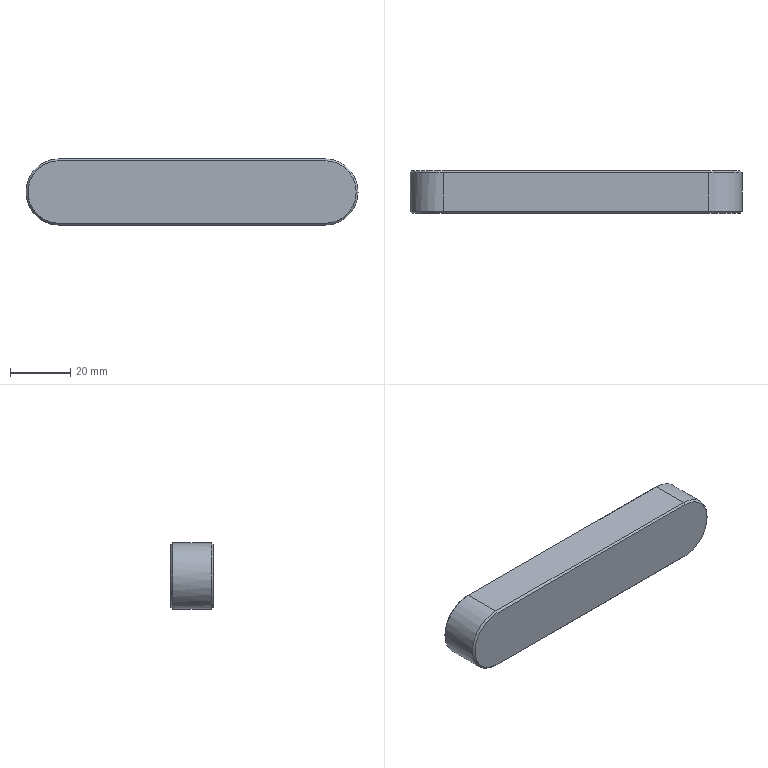Part | STEP file | Input 104 | 1 solid | 17 faces | box 110 x 14 x 22 mm | volume 32338 mm3 | plane 8 | cone 6 | cylinder 3 | commonest cylinder face diameters 22 x3
STEP:
#1=CARTESIAN_POINT('',(0.,0.,0.));
#2=DIRECTION('',(0.,0.,1.));
#3=DIRECTION('',(1.,0.,0.));
#4=AXIS2_PLACEMENT_3D('',#1,#2,#3);
#5=CARTESIAN_POINT('',(4274.4,696.,-0.4063));
#6=VERTEX_POINT('',#5);
#7=CARTESIAN_POINT('',(4264.,696.,9.994));
#8=VERTEX_POINT('',#7);
#9=CARTESIAN_POINT('',(4264.,696.,-0.4063));
#10=DIRECTION('',(0.,-1.,0.));
#11=DIRECTION('',(-1.,0.,0.));
#12=AXIS2_PLACEMENT_3D('',#9,#10,#11);
#13=CIRCLE('',#12,10.4);
#14=CARTESIAN_POINT('',(4264.,696.,-0.4063));
#15=DIRECTION('',(0.,1.,0.));
#16=DIRECTION('',(1.,0.,0.));
#17=AXIS2_PLACEMENT_3D('',#14,#15,#16);
#18=CONICAL_SURFACE('',#17,10.4,0.7854);
#19=CARTESIAN_POINT('',(9.425,0.));
#20=DIRECTION('',(-1.,0.));
#21=VECTOR('',#20,1.);
#22=LINE('',#19,#21);
#23=(GEOMETRIC_REPRESENTATION_CONTEXT(2)PARAMETRIC_REPRESENTATION_CONTEXT()REPRESENTATION_CONTEXT('',''));
#24=DEFINITIONAL_REPRESENTATION('',(#22),#23);
#25=PCURVE('',#18,#24);
#26=CARTESIAN_POINT('',(4220.,696.,-0.4063));
#27=DIRECTION('',(0.,-1.,0.));
#28=DIRECTION('',(-1.,0.,0.));
#29=AXIS2_PLACEMENT_3D('',#26,#27,#28);
#30=PLANE('',#29);
#31=CARTESIAN_POINT('',(-44.,0.));
#32=DIRECTION('',(1.,0.));
#33=AXIS2_PLACEMENT_2D('',#31,#32);
#34=CIRCLE('',#33,10.4);
#35=(GEOMETRIC_REPRESENTATION_CONTEXT(2)PARAMETRIC_REPRESENTATION_CONTEXT()REPRESENTATION_CONTEXT('',''));
#36=DEFINITIONAL_REPRESENTATION('',(#34),#35);
#37=PCURVE('',#30,#36);
#38=SURFACE_CURVE('',#13,(#25,#37),.PCURVE_S1.);
#39=EDGE_CURVE('',#6,#8,#38,.T.);
#40=ORIENTED_EDGE('',*,*,#39,.F.);
#41=CARTESIAN_POINT('',(4275.,696.6,-0.4063));
#42=VERTEX_POINT('',#41);
#43=CARTESIAN_POINT('',(4274.4,696.,-0.4063));
#44=DIRECTION('',(0.7071,0.7071,0.));
#45=VECTOR('',#44,1.);
#46=LINE('',#43,#45);
#47=CARTESIAN_POINT('',(6.283,0.));
#48=DIRECTION('',(0.,1.));
#49=VECTOR('',#48,1.);
#50=LINE('',#47,#49);
#51=(GEOMETRIC_REPRESENTATION_CONTEXT(2)PARAMETRIC_REPRESENTATION_CONTEXT()REPRESENTATION_CONTEXT('',''));
#52=DEFINITIONAL_REPRESENTATION('',(#50),#51);
#53=PCURVE('',#18,#52);
#54=CARTESIAN_POINT('',(4264.,696.,-0.4063));
#55=DIRECTION('',(0.,1.,0.));
#56=DIRECTION('',(1.,0.,0.));
#57=AXIS2_PLACEMENT_3D('',#54,#55,#56);
#58=CONICAL_SURFACE('',#57,10.4,0.7854);
#59=CARTESIAN_POINT('',(0.,0.));
#60=DIRECTION('',(0.,1.));
#61=VECTOR('',#60,1.);
#62=LINE('',#59,#61);
#63=(GEOMETRIC_REPRESENTATION_CONTEXT(2)PARAMETRIC_REPRESENTATION_CONTEXT()REPRESENTATION_CONTEXT('',''));
#64=DEFINITIONAL_REPRESENTATION('',(#62),#63);
#65=PCURVE('',#58,#64);
#66=SURFACE_CURVE('',#46,(#53,#65),.PCURVE_S1.);
#67=EDGE_CURVE('',#6,#42,#66,.T.);
#68=ORIENTED_EDGE('',*,*,#67,.T.);
#69=CARTESIAN_POINT('',(4264.,696.6,10.594));
#70=VERTEX_POINT('',#69);
#71=CARTESIAN_POINT('',(4264.,696.6,-0.4063));
#72=DIRECTION('',(0.,1.,0.));
#73=DIRECTION('',(-1.,0.,0.));
#74=AXIS2_PLACEMENT_3D('',#71,#72,#73);
#75=CIRCLE('',#74,11.);
#76=CARTESIAN_POINT('',(3.142,0.6));
#77=DIRECTION('',(1.,0.));
#78=VECTOR('',#77,1.);
#79=LINE('',#76,#78);
#80=(GEOMETRIC_REPRESENTATION_CONTEXT(2)PARAMETRIC_REPRESENTATION_CONTEXT()REPRESENTATION_CONTEXT('',''));
#81=DEFINITIONAL_REPRESENTATION('',(#79),#80);
#82=PCURVE('',#18,#81);
#83=CARTESIAN_POINT('',(4264.,696.,-0.4063));
#84=DIRECTION('',(0.,1.,0.));
#85=DIRECTION('',(1.,0.,0.));
#86=AXIS2_PLACEMENT_3D('',#83,#84,#85);
#87=CYLINDRICAL_SURFACE('',#86,11.);
#88=CARTESIAN_POINT('',(3.142,0.6));
#89=DIRECTION('',(1.,0.));
#90=VECTOR('',#89,1.);
#91=LINE('',#88,#90);
#92=(GEOMETRIC_REPRESENTATION_CONTEXT(2)PARAMETRIC_REPRESENTATION_CONTEXT()REPRESENTATION_CONTEXT('',''));
#93=DEFINITIONAL_REPRESENTATION('',(#91),#92);
#94=PCURVE('',#87,#93);
#95=SURFACE_CURVE('',#75,(#82,#94),.PCURVE_S1.);
#96=EDGE_CURVE('',#70,#42,#95,.T.);
#97=ORIENTED_EDGE('',*,*,#96,.F.);
#98=CARTESIAN_POINT('',(4264.,696.,9.994));
#99=DIRECTION('',(0.,0.7071,0.7071));
#100=VECTOR('',#99,1.);
#101=LINE('',#98,#100);
#102=CARTESIAN_POINT('',(4.712,0.));
#103=DIRECTION('',(0.,1.));
#104=VECTOR('',#103,1.);
#105=LINE('',#102,#104);
#106=(GEOMETRIC_REPRESENTATION_CONTEXT(2)PARAMETRIC_REPRESENTATION_CONTEXT()REPRESENTATION_CONTEXT('',''));
#107=DEFINITIONAL_REPRESENTATION('',(#105),#106);
#108=PCURVE('',#18,#107);
#109=CARTESIAN_POINT('',(4220.,696.6,10.594));
#110=DIRECTION('',(0.,0.7071,-0.7071));
#111=DIRECTION('',(0.,0.7071,0.7071));
#112=AXIS2_PLACEMENT_3D('',#109,#110,#111);
#113=PLANE('',#112);
#114=CARTESIAN_POINT('',(-0.8485,44.));
#115=DIRECTION('',(1.,0.));
#116=VECTOR('',#115,1.);
#117=LINE('',#114,#116);
#118=(GEOMETRIC_REPRESENTATION_CONTEXT(2)PARAMETRIC_REPRESENTATION_CONTEXT()REPRESENTATION_CONTEXT('',''));
#119=DEFINITIONAL_REPRESENTATION('',(#117),#118);
#120=PCURVE('',#113,#119);
#121=SURFACE_CURVE('',#101,(#108,#120),.PCURVE_S1.);
#122=EDGE_CURVE('',#8,#70,#121,.T.);
#123=ORIENTED_EDGE('',*,*,#122,.F.);
#124=EDGE_LOOP('',(#40,#68,#97,#123));
#125=FACE_BOUND('',#124,.T.);
#126=ADVANCED_FACE('',(#125),#18,.T.);
#127=CARTESIAN_POINT('',(4165.6,710.,-0.4063));
#128=VERTEX_POINT('',#127);
#129=CARTESIAN_POINT('',(4176.,710.,9.994));
#130=VERTEX_POINT('',#129);
#131=CARTESIAN_POINT('',(4176.,710.,-0.4063));
#132=DIRECTION('',(0.,1.,0.));
#133=DIRECTION('',(1.,0.,0.));
#134=AXIS2_PLACEMENT_3D('',#131,#132,#133);
#135=CIRCLE('',#134,10.4);
#136=CARTESIAN_POINT('',(4176.,710.,-0.4063));
#137=DIRECTION('',(0.,-1.,0.));
#138=DIRECTION('',(-1.,0.,0.));
#139=AXIS2_PLACEMENT_3D('',#136,#137,#138);
#140=CONICAL_SURFACE('',#139,10.4,0.7854);
#141=CARTESIAN_POINT('',(9.425,0.));
#142=DIRECTION('',(-1.,0.));
#143=VECTOR('',#142,1.);
#144=LINE('',#141,#143);
#145=(GEOMETRIC_REPRESENTATION_CONTEXT(2)PARAMETRIC_REPRESENTATION_CONTEXT()REPRESENTATION_CONTEXT('',''));
#146=DEFINITIONAL_REPRESENTATION('',(#144),#145);
#147=PCURVE('',#140,#146);
#148=CARTESIAN_POINT('',(4220.,710.,-0.4063));
#149=DIRECTION('',(0.,1.,0.));
#150=DIRECTION('',(1.,0.,0.));
#151=AXIS2_PLACEMENT_3D('',#148,#149,#150);
#152=PLANE('',#151);
#153=CARTESIAN_POINT('',(-44.,0.));
#154=DIRECTION('',(1.,0.));
#155=AXIS2_PLACEMENT_2D('',#153,#154);
#156=CIRCLE('',#155,10.4);
#157=(GEOMETRIC_REPRESENTATION_CONTEXT(2)PARAMETRIC_REPRESENTATION_CONTEXT()REPRESENTATION_CONTEXT('',''));
#158=DEFINITIONAL_REPRESENTATION('',(#156),#157);
#159=PCURVE('',#152,#158);
#160=SURFACE_CURVE('',#135,(#147,#159),.PCURVE_S1.);
#161=EDGE_CURVE('',#128,#130,#160,.T.);
#162=ORIENTED_EDGE('',*,*,#161,.F.);
#163=CARTESIAN_POINT('',(4165.,709.4,-0.4063));
#164=VERTEX_POINT('',#163);
#165=CARTESIAN_POINT('',(4165.6,710.,-0.4063));
#166=DIRECTION('',(-0.7071,-0.7071,0.));
#167=VECTOR('',#166,1.);
#168=LINE('',#165,#167);
#169=CARTESIAN_POINT('',(6.283,0.));
#170=DIRECTION('',(0.,1.));
#171=VECTOR('',#170,1.);
#172=LINE('',#169,#171);
#173=(GEOMETRIC_REPRESENTATION_CONTEXT(2)PARAMETRIC_REPRESENTATION_CONTEXT()REPRESENTATION_CONTEXT('',''));
#174=DEFINITIONAL_REPRESENTATION('',(#172),#173);
#175=PCURVE('',#140,#174);
#176=CARTESIAN_POINT('',(4176.,710.,-0.4063));
#177=DIRECTION('',(0.,-1.,0.));
#178=DIRECTION('',(-1.,0.,0.));
#179=AXIS2_PLACEMENT_3D('',#176,#177,#178);
#180=CONICAL_SURFACE('',#179,10.4,0.7854);
#181=CARTESIAN_POINT('',(0.,0.));
#182=DIRECTION('',(0.,1.));
#183=VECTOR('',#182,1.);
#184=LINE('',#181,#183);
#185=(GEOMETRIC_REPRESENTATION_CONTEXT(2)PARAMETRIC_REPRESENTATION_CONTEXT()REPRESENTATION_CONTEXT('',''));
#186=DEFINITIONAL_REPRESENTATION('',(#184),#185);
#187=PCURVE('',#180,#186);
#188=SURFACE_CURVE('',#168,(#175,#187),.PCURVE_S1.);
#189=EDGE_CURVE('',#128,#164,#188,.T.);
#190=ORIENTED_EDGE('',*,*,#189,.T.);
#191=CARTESIAN_POINT('',(4176.,709.4,10.594));
#192=VERTEX_POINT('',#191);
#193=CARTESIAN_POINT('',(4176.,709.4,-0.4063));
#194=DIRECTION('',(0.,-1.,0.));
#195=DIRECTION('',(1.,0.,0.));
#196=AXIS2_PLACEMENT_3D('',#193,#194,#195);
#197=CIRCLE('',#196,11.);
#198=CARTESIAN_POINT('',(3.142,0.6));
#199=DIRECTION('',(1.,0.));
#200=VECTOR('',#199,1.);
#201=LINE('',#198,#200);
#202=(GEOMETRIC_REPRESENTATION_CONTEXT(2)PARAMETRIC_REPRESENTATION_CONTEXT()REPRESENTATION_CONTEXT('',''));
#203=DEFINITIONAL_REPRESENTATION('',(#201),#202);
#204=PCURVE('',#140,#203);
#205=CARTESIAN_POINT('',(4176.,696.,-0.4063));
#206=DIRECTION('',(0.,1.,0.));
#207=DIRECTION('',(1.,0.,0.));
#208=AXIS2_PLACEMENT_3D('',#205,#206,#207);
#209=CYLINDRICAL_SURFACE('',#208,11.);
#210=CARTESIAN_POINT('',(6.283,13.4));
#211=DIRECTION('',(-1.,0.));
#212=VECTOR('',#211,1.);
#213=LINE('',#210,#212);
#214=(GEOMETRIC_REPRESENTATION_CONTEXT(2)PARAMETRIC_REPRESENTATION_CONTEXT()REPRESENTATION_CONTEXT('',''));
#215=DEFINITIONAL_REPRESENTATION('',(#213),#214);
#216=PCURVE('',#209,#215);
#217=SURFACE_CURVE('',#197,(#204,#216),.PCURVE_S1.);
#218=EDGE_CURVE('',#192,#164,#217,.T.);
#219=ORIENTED_EDGE('',*,*,#218,.F.);
#220=CARTESIAN_POINT('',(4176.,709.4,10.594));
#221=DIRECTION('',(0.,0.7071,-0.7071));
#222=VECTOR('',#221,1.);
#223=LINE('',#220,#222);
#224=CARTESIAN_POINT('',(4.712,0.6));
#225=DIRECTION('',(0.,-1.));
#226=VECTOR('',#225,1.);
#227=LINE('',#224,#226);
#228=(GEOMETRIC_REPRESENTATION_CONTEXT(2)PARAMETRIC_REPRESENTATION_CONTEXT()REPRESENTATION_CONTEXT('',''));
#229=DEFINITIONAL_REPRESENTATION('',(#227),#228);
#230=PCURVE('',#140,#229);
#231=CARTESIAN_POINT('',(4220.,709.4,10.594));
#232=DIRECTION('',(0.,-0.7071,-0.7071));
#233=DIRECTION('',(0.,0.7071,-0.7071));
#234=AXIS2_PLACEMENT_3D('',#231,#232,#233);
#235=PLANE('',#234);
#236=CARTESIAN_POINT('',(0.,-44.));
#237=DIRECTION('',(1.,0.));
#238=VECTOR('',#237,1.);
#239=LINE('',#236,#238);
#240=(GEOMETRIC_REPRESENTATION_CONTEXT(2)PARAMETRIC_REPRESENTATION_CONTEXT()REPRESENTATION_CONTEXT('',''));
#241=DEFINITIONAL_REPRESENTATION('',(#239),#240);
#242=PCURVE('',#235,#241);
#243=SURFACE_CURVE('',#223,(#230,#242),.PCURVE_S1.);
#244=EDGE_CURVE('',#192,#130,#243,.T.);
#245=ORIENTED_EDGE('',*,*,#244,.T.);
#246=EDGE_LOOP('',(#162,#190,#219,#245));
#247=FACE_BOUND('',#246,.T.);
#248=ADVANCED_FACE('',(#247),#140,.T.);
#249=ORIENTED_EDGE('',*,*,#96,.T.);
#250=CARTESIAN_POINT('',(4275.,709.4,-0.4063));
#251=VERTEX_POINT('',#250);
#252=CARTESIAN_POINT('',(4275.,696.,-0.4063));
#253=DIRECTION('',(0.,1.,0.));
#254=VECTOR('',#253,1.);
#255=LINE('',#252,#254);
#256=CARTESIAN_POINT('',(6.283,0.));
#257=DIRECTION('',(0.,1.));
#258=VECTOR('',#257,1.);
#259=LINE('',#256,#258);
#260=(GEOMETRIC_REPRESENTATION_CONTEXT(2)PARAMETRIC_REPRESENTATION_CONTEXT()REPRESENTATION_CONTEXT('',''));
#261=DEFINITIONAL_REPRESENTATION('',(#259),#260);
#262=PCURVE('',#87,#261);
#263=CARTESIAN_POINT('',(4264.,696.,-0.4063));
#264=DIRECTION('',(0.,1.,0.));
#265=DIRECTION('',(1.,0.,0.));
#266=AXIS2_PLACEMENT_3D('',#263,#264,#265);
#267=CYLINDRICAL_SURFACE('',#266,11.);
#268=CARTESIAN_POINT('',(0.,0.));
#269=DIRECTION('',(0.,1.));
#270=VECTOR('',#269,1.);
#271=LINE('',#268,#270);
#272=(GEOMETRIC_REPRESENTATION_CONTEXT(2)PARAMETRIC_REPRESENTATION_CONTEXT()REPRESENTATION_CONTEXT('',''));
#273=DEFINITIONAL_REPRESENTATION('',(#271),#272);
#274=PCURVE('',#267,#273);
#275=SURFACE_CURVE('',#255,(#262,#274),.PCURVE_S1.);
#276=EDGE_CURVE('',#42,#251,#275,.T.);
#277=ORIENTED_EDGE('',*,*,#276,.T.);
#278=CARTESIAN_POINT('',(4264.,709.4,10.594));
#279=VERTEX_POINT('',#278);
#280=CARTESIAN_POINT('',(4264.,709.4,-0.4063));
#281=DIRECTION('',(0.,-1.,0.));
#282=DIRECTION('',(1.,0.,0.));
#283=AXIS2_PLACEMENT_3D('',#280,#281,#282);
#284=CIRCLE('',#283,11.);
#285=CARTESIAN_POINT('',(6.283,13.4));
#286=DIRECTION('',(-1.,0.));
#287=VECTOR('',#286,1.);
#288=LINE('',#285,#287);
#289=(GEOMETRIC_REPRESENTATION_CONTEXT(2)PARAMETRIC_REPRESENTATION_CONTEXT()REPRESENTATION_CONTEXT('',''));
#290=DEFINITIONAL_REPRESENTATION('',(#288),#289);
#291=PCURVE('',#87,#290);
#292=CARTESIAN_POINT('',(4264.,710.,-0.4063));
#293=DIRECTION('',(0.,-1.,0.));
#294=DIRECTION('',(-1.,0.,0.));
#295=AXIS2_PLACEMENT_3D('',#292,#293,#294);
#296=CONICAL_SURFACE('',#295,10.4,0.7854);
#297=CARTESIAN_POINT('',(3.142,0.6));
#298=DIRECTION('',(1.,0.));
#299=VECTOR('',#298,1.);
#300=LINE('',#297,#299);
#301=(GEOMETRIC_REPRESENTATION_CONTEXT(2)PARAMETRIC_REPRESENTATION_CONTEXT()REPRESENTATION_CONTEXT('',''));
#302=DEFINITIONAL_REPRESENTATION('',(#300),#301);
#303=PCURVE('',#296,#302);
#304=SURFACE_CURVE('',#284,(#291,#303),.PCURVE_S1.);
#305=EDGE_CURVE('',#251,#279,#304,.T.);
#306=ORIENTED_EDGE('',*,*,#305,.T.);
#307=CARTESIAN_POINT('',(4264.,696.,10.594));
#308=DIRECTION('',(0.,1.,0.));
#309=VECTOR('',#308,1.);
#310=LINE('',#307,#309);
#311=CARTESIAN_POINT('',(4.712,0.));
#312=DIRECTION('',(0.,1.));
#313=VECTOR('',#312,1.);
#314=LINE('',#311,#313);
#315=(GEOMETRIC_REPRESENTATION_CONTEXT(2)PARAMETRIC_REPRESENTATION_CONTEXT()REPRESENTATION_CONTEXT('',''));
#316=DEFINITIONAL_REPRESENTATION('',(#314),#315);
#317=PCURVE('',#87,#316);
#318=CARTESIAN_POINT('',(4220.,696.,10.594));
#319=DIRECTION('',(0.,0.,1.));
#320=DIRECTION('',(0.,-1.,0.));
#321=AXIS2_PLACEMENT_3D('',#318,#319,#320);
#322=PLANE('',#321);
#323=CARTESIAN_POINT('',(0.,44.));
#324=DIRECTION('',(-1.,0.));
#325=VECTOR('',#324,1.);
#326=LINE('',#323,#325);
#327=(GEOMETRIC_REPRESENTATION_CONTEXT(2)PARAMETRIC_REPRESENTATION_CONTEXT()REPRESENTATION_CONTEXT('',''));
#328=DEFINITIONAL_REPRESENTATION('',(#326),#327);
#329=PCURVE('',#322,#328);
#330=SURFACE_CURVE('',#310,(#317,#329),.PCURVE_S1.);
#331=EDGE_CURVE('',#70,#279,#330,.T.);
#332=ORIENTED_EDGE('',*,*,#331,.F.);
#333=EDGE_LOOP('',(#249,#277,#306,#332));
#334=FACE_BOUND('',#333,.T.);
#335=ADVANCED_FACE('',(#334),#87,.T.);
#336=CARTESIAN_POINT('',(4264.,710.,-10.806));
#337=VERTEX_POINT('',#336);
#338=CARTESIAN_POINT('',(4176.,710.,-10.806));
#339=VERTEX_POINT('',#338);
#340=CARTESIAN_POINT('',(4220.,710.,-10.806));
#341=DIRECTION('',(-1.,0.,0.));
#342=VECTOR('',#341,1.);
#343=LINE('',#340,#342);
#344=CARTESIAN_POINT('',(0.,10.4));
#345=DIRECTION('',(-1.,0.));
#346=VECTOR('',#345,1.);
#347=LINE('',#344,#346);
#348=(GEOMETRIC_REPRESENTATION_CONTEXT(2)PARAMETRIC_REPRESENTATION_CONTEXT()REPRESENTATION_CONTEXT('',''));
#349=DEFINITIONAL_REPRESENTATION('',(#347),#348);
#350=PCURVE('',#152,#349);
#351=CARTESIAN_POINT('',(4220.,709.4,-11.406));
#352=DIRECTION('',(0.,-0.7071,0.7071));
#353=DIRECTION('',(0.,-0.7071,-0.7071));
#354=AXIS2_PLACEMENT_3D('',#351,#352,#353);
#355=PLANE('',#354);
#356=CARTESIAN_POINT('',(-0.8485,0.));
#357=DIRECTION('',(0.,-1.));
#358=VECTOR('',#357,1.);
#359=LINE('',#356,#358);
#360=(GEOMETRIC_REPRESENTATION_CONTEXT(2)PARAMETRIC_REPRESENTATION_CONTEXT()REPRESENTATION_CONTEXT('',''));
#361=DEFINITIONAL_REPRESENTATION('',(#359),#360);
#362=PCURVE('',#355,#361);
#363=SURFACE_CURVE('',#343,(#350,#362),.PCURVE_S1.);
#364=EDGE_CURVE('',#337,#339,#363,.T.);
#365=ORIENTED_EDGE('',*,*,#364,.T.);
#366=CARTESIAN_POINT('',(4176.,710.,-0.4063));
#367=DIRECTION('',(0.,1.,0.));
#368=DIRECTION('',(1.,0.,0.));
#369=AXIS2_PLACEMENT_3D('',#366,#367,#368);
#370=CIRCLE('',#369,10.4);
#371=CARTESIAN_POINT('',(-44.,0.));
#372=DIRECTION('',(1.,0.));
#373=AXIS2_PLACEMENT_2D('',#371,#372);
#374=CIRCLE('',#373,10.4);
#375=(GEOMETRIC_REPRESENTATION_CONTEXT(2)PARAMETRIC_REPRESENTATION_CONTEXT()REPRESENTATION_CONTEXT('',''));
#376=DEFINITIONAL_REPRESENTATION('',(#374),#375);
#377=PCURVE('',#152,#376);
#378=CARTESIAN_POINT('',(3.142,0.));
#379=DIRECTION('',(-1.,0.));
#380=VECTOR('',#379,1.);
#381=LINE('',#378,#380);
#382=(GEOMETRIC_REPRESENTATION_CONTEXT(2)PARAMETRIC_REPRESENTATION_CONTEXT()REPRESENTATION_CONTEXT('',''));
#383=DEFINITIONAL_REPRESENTATION('',(#381),#382);
#384=PCURVE('',#180,#383);
#385=SURFACE_CURVE('',#370,(#377,#384),.PCURVE_S1.);
#386=EDGE_CURVE('',#339,#128,#385,.T.);
#387=ORIENTED_EDGE('',*,*,#386,.T.);
#388=ORIENTED_EDGE('',*,*,#161,.T.);
#389=CARTESIAN_POINT('',(4264.,710.,9.994));
#390=VERTEX_POINT('',#389);
#391=CARTESIAN_POINT('',(4220.,710.,9.994));
#392=DIRECTION('',(1.,0.,0.));
#393=VECTOR('',#392,1.);
#394=LINE('',#391,#393);
#395=CARTESIAN_POINT('',(0.,-10.4));
#396=DIRECTION('',(1.,0.));
#397=VECTOR('',#396,1.);
#398=LINE('',#395,#397);
#399=(GEOMETRIC_REPRESENTATION_CONTEXT(2)PARAMETRIC_REPRESENTATION_CONTEXT()REPRESENTATION_CONTEXT('',''));
#400=DEFINITIONAL_REPRESENTATION('',(#398),#399);
#401=PCURVE('',#152,#400);
#402=CARTESIAN_POINT('',(0.8485,0.));
#403=DIRECTION('',(0.,1.));
#404=VECTOR('',#403,1.);
#405=LINE('',#402,#404);
#406=(GEOMETRIC_REPRESENTATION_CONTEXT(2)PARAMETRIC_REPRESENTATION_CONTEXT()REPRESENTATION_CONTEXT('',''));
#407=DEFINITIONAL_REPRESENTATION('',(#405),#406);
#408=PCURVE('',#235,#407);
#409=SURFACE_CURVE('',#394,(#401,#408),.PCURVE_S1.);
#410=EDGE_CURVE('',#130,#390,#409,.T.);
#411=ORIENTED_EDGE('',*,*,#410,.T.);
#412=CARTESIAN_POINT('',(4264.,710.,-0.4063));
#413=DIRECTION('',(0.,1.,0.));
#414=DIRECTION('',(1.,0.,0.));
#415=AXIS2_PLACEMENT_3D('',#412,#413,#414);
#416=CIRCLE('',#415,10.4);
#417=CARTESIAN_POINT('',(44.,0.));
#418=DIRECTION('',(1.,0.));
#419=AXIS2_PLACEMENT_2D('',#417,#418);
#420=CIRCLE('',#419,10.4);
#421=(GEOMETRIC_REPRESENTATION_CONTEXT(2)PARAMETRIC_REPRESENTATION_CONTEXT()REPRESENTATION_CONTEXT('',''));
#422=DEFINITIONAL_REPRESENTATION('',(#420),#421);
#423=PCURVE('',#152,#422);
#424=CARTESIAN_POINT('',(9.425,0.));
#425=DIRECTION('',(-1.,0.));
#426=VECTOR('',#425,1.);
#427=LINE('',#424,#426);
#428=(GEOMETRIC_REPRESENTATION_CONTEXT(2)PARAMETRIC_REPRESENTATION_CONTEXT()REPRESENTATION_CONTEXT('',''));
#429=DEFINITIONAL_REPRESENTATION('',(#427),#428);
#430=PCURVE('',#296,#429);
#431=SURFACE_CURVE('',#416,(#423,#430),.PCURVE_S1.);
#432=EDGE_CURVE('',#390,#337,#431,.T.);
#433=ORIENTED_EDGE('',*,*,#432,.T.);
#434=EDGE_LOOP('',(#365,#387,#388,#411,#433));
#435=FACE_BOUND('',#434,.T.);
#436=ADVANCED_FACE('',(#435),#152,.T.);
#437=CARTESIAN_POINT('',(4176.,696.6,10.594));
#438=VERTEX_POINT('',#437);
#439=CARTESIAN_POINT('',(4176.,696.,10.594));
#440=DIRECTION('',(0.,-1.,0.));
#441=VECTOR('',#440,1.);
#442=LINE('',#439,#441);
#443=CARTESIAN_POINT('',(0.,-44.));
#444=DIRECTION('',(1.,0.));
#445=VECTOR('',#444,1.);
#446=LINE('',#443,#445);
#447=(GEOMETRIC_REPRESENTATION_CONTEXT(2)PARAMETRIC_REPRESENTATION_CONTEXT()REPRESENTATION_CONTEXT('',''));
#448=DEFINITIONAL_REPRESENTATION('',(#446),#447);
#449=PCURVE('',#322,#448);
#450=CARTESIAN_POINT('',(4.712,0.));
#451=DIRECTION('',(0.,-1.));
#452=VECTOR('',#451,1.);
#453=LINE('',#450,#452);
#454=(GEOMETRIC_REPRESENTATION_CONTEXT(2)PARAMETRIC_REPRESENTATION_CONTEXT()REPRESENTATION_CONTEXT('',''));
#455=DEFINITIONAL_REPRESENTATION('',(#453),#454);
#456=PCURVE('',#209,#455);
#457=SURFACE_CURVE('',#442,(#449,#456),.PCURVE_S1.);
#458=EDGE_CURVE('',#192,#438,#457,.T.);
#459=ORIENTED_EDGE('',*,*,#458,.T.);
#460=CARTESIAN_POINT('',(4220.,696.6,10.594));
#461=DIRECTION('',(1.,0.,0.));
#462=VECTOR('',#461,1.);
#463=LINE('',#460,#462);
#464=CARTESIAN_POINT('',(-0.6,0.));
#465=DIRECTION('',(0.,1.));
#466=VECTOR('',#465,1.);
#467=LINE('',#464,#466);
#468=(GEOMETRIC_REPRESENTATION_CONTEXT(2)PARAMETRIC_REPRESENTATION_CONTEXT()REPRESENTATION_CONTEXT('',''));
#469=DEFINITIONAL_REPRESENTATION('',(#467),#468);
#470=PCURVE('',#322,#469);
#471=CARTESIAN_POINT('',(0.,0.));
#472=DIRECTION('',(0.,1.));
#473=VECTOR('',#472,1.);
#474=LINE('',#471,#473);
#475=(GEOMETRIC_REPRESENTATION_CONTEXT(2)PARAMETRIC_REPRESENTATION_CONTEXT()REPRESENTATION_CONTEXT('',''));
#476=DEFINITIONAL_REPRESENTATION('',(#474),#475);
#477=PCURVE('',#113,#476);
#478=SURFACE_CURVE('',#463,(#470,#477),.PCURVE_S1.);
#479=EDGE_CURVE('',#438,#70,#478,.T.);
#480=ORIENTED_EDGE('',*,*,#479,.T.);
#481=ORIENTED_EDGE('',*,*,#331,.T.);
#482=CARTESIAN_POINT('',(4220.,709.4,10.594));
#483=DIRECTION('',(-1.,0.,0.));
#484=VECTOR('',#483,1.);
#485=LINE('',#482,#484);
#486=CARTESIAN_POINT('',(-13.4,0.));
#487=DIRECTION('',(0.,-1.));
#488=VECTOR('',#487,1.);
#489=LINE('',#486,#488);
#490=(GEOMETRIC_REPRESENTATION_CONTEXT(2)PARAMETRIC_REPRESENTATION_CONTEXT()REPRESENTATION_CONTEXT('',''));
#491=DEFINITIONAL_REPRESENTATION('',(#489),#490);
#492=PCURVE('',#322,#491);
#493=CARTESIAN_POINT('',(0.,0.));
#494=DIRECTION('',(0.,-1.));
#495=VECTOR('',#494,1.);
#496=LINE('',#493,#495);
#497=(GEOMETRIC_REPRESENTATION_CONTEXT(2)PARAMETRIC_REPRESENTATION_CONTEXT()REPRESENTATION_CONTEXT('',''));
#498=DEFINITIONAL_REPRESENTATION('',(#496),#497);
#499=PCURVE('',#235,#498);
#500=SURFACE_CURVE('',#485,(#492,#499),.PCURVE_S1.);
#501=EDGE_CURVE('',#279,#192,#500,.T.);
#502=ORIENTED_EDGE('',*,*,#501,.T.);
#503=EDGE_LOOP('',(#459,#480,#481,#502));
#504=FACE_BOUND('',#503,.T.);
#505=ADVANCED_FACE('',(#504),#322,.T.);
#506=CARTESIAN_POINT('',(4264.,709.4,-11.406));
#507=VERTEX_POINT('',#506);
#508=CARTESIAN_POINT('',(4264.,696.6,-11.406));
#509=VERTEX_POINT('',#508);
#510=CARTESIAN_POINT('',(4264.,696.,-11.406));
#511=DIRECTION('',(0.,-1.,0.));
#512=VECTOR('',#511,1.);
#513=LINE('',#510,#512);
#514=CARTESIAN_POINT('',(4220.,696.,-11.406));
#515=DIRECTION('',(0.,0.,-1.));
#516=DIRECTION('',(0.,1.,0.));
#517=AXIS2_PLACEMENT_3D('',#514,#515,#516);
#518=PLANE('',#517);
#519=CARTESIAN_POINT('',(0.,44.));
#520=DIRECTION('',(-1.,0.));
#521=VECTOR('',#520,1.);
#522=LINE('',#519,#521);
#523=(GEOMETRIC_REPRESENTATION_CONTEXT(2)PARAMETRIC_REPRESENTATION_CONTEXT()REPRESENTATION_CONTEXT('',''));
#524=DEFINITIONAL_REPRESENTATION('',(#522),#523);
#525=PCURVE('',#518,#524);
#526=CARTESIAN_POINT('',(1.571,0.));
#527=DIRECTION('',(0.,-1.));
#528=VECTOR('',#527,1.);
#529=LINE('',#526,#528);
#530=(GEOMETRIC_REPRESENTATION_CONTEXT(2)PARAMETRIC_REPRESENTATION_CONTEXT()REPRESENTATION_CONTEXT('',''));
#531=DEFINITIONAL_REPRESENTATION('',(#529),#530);
#532=PCURVE('',#267,#531);
#533=SURFACE_CURVE('',#513,(#525,#532),.PCURVE_S1.);
#534=EDGE_CURVE('',#507,#509,#533,.T.);
#535=ORIENTED_EDGE('',*,*,#534,.T.);
#536=CARTESIAN_POINT('',(4176.,696.6,-11.406));
#537=VERTEX_POINT('',#536);
#538=CARTESIAN_POINT('',(4220.,696.6,-11.406));
#539=DIRECTION('',(-1.,0.,0.));
#540=VECTOR('',#539,1.);
#541=LINE('',#538,#540);
#542=CARTESIAN_POINT('',(0.6,0.));
#543=DIRECTION('',(0.,-1.));
#544=VECTOR('',#543,1.);
#545=LINE('',#542,#544);
#546=(GEOMETRIC_REPRESENTATION_CONTEXT(2)PARAMETRIC_REPRESENTATION_CONTEXT()REPRESENTATION_CONTEXT('',''));
#547=DEFINITIONAL_REPRESENTATION('',(#545),#546);
#548=PCURVE('',#518,#547);
#549=CARTESIAN_POINT('',(4220.,696.6,-11.406));
#550=DIRECTION('',(0.,0.7071,0.7071));
#551=DIRECTION('',(0.,-0.7071,0.7071));
#552=AXIS2_PLACEMENT_3D('',#549,#550,#551);
#553=PLANE('',#552);
#554=CARTESIAN_POINT('',(0.,0.));
#555=DIRECTION('',(0.,-1.));
#556=VECTOR('',#555,1.);
#557=LINE('',#554,#556);
#558=(GEOMETRIC_REPRESENTATION_CONTEXT(2)PARAMETRIC_REPRESENTATION_CONTEXT()REPRESENTATION_CONTEXT('',''));
#559=DEFINITIONAL_REPRESENTATION('',(#557),#558);
#560=PCURVE('',#553,#559);
#561=SURFACE_CURVE('',#541,(#548,#560),.PCURVE_S1.);
#562=EDGE_CURVE('',#509,#537,#561,.T.);
#563=ORIENTED_EDGE('',*,*,#562,.T.);
#564=CARTESIAN_POINT('',(4176.,709.4,-11.406));
#565=VERTEX_POINT('',#564);
#566=CARTESIAN_POINT('',(4176.,696.,-11.406));
#567=DIRECTION('',(0.,1.,0.));
#568=VECTOR('',#567,1.);
#569=LINE('',#566,#568);
#570=CARTESIAN_POINT('',(0.,-44.));
#571=DIRECTION('',(1.,0.));
#572=VECTOR('',#571,1.);
#573=LINE('',#570,#572);
#574=(GEOMETRIC_REPRESENTATION_CONTEXT(2)PARAMETRIC_REPRESENTATION_CONTEXT()REPRESENTATION_CONTEXT('',''));
#575=DEFINITIONAL_REPRESENTATION('',(#573),#574);
#576=PCURVE('',#518,#575);
#577=CARTESIAN_POINT('',(1.571,0.));
#578=DIRECTION('',(0.,1.));
#579=VECTOR('',#578,1.);
#580=LINE('',#577,#579);
#581=(GEOMETRIC_REPRESENTATION_CONTEXT(2)PARAMETRIC_REPRESENTATION_CONTEXT()REPRESENTATION_CONTEXT('',''));
#582=DEFINITIONAL_REPRESENTATION('',(#580),#581);
#583=PCURVE('',#209,#582);
#584=SURFACE_CURVE('',#569,(#576,#583),.PCURVE_S1.);
#585=EDGE_CURVE('',#537,#565,#584,.T.);
#586=ORIENTED_EDGE('',*,*,#585,.T.);
#587=CARTESIAN_POINT('',(4220.,709.4,-11.406));
#588=DIRECTION('',(1.,0.,0.));
#589=VECTOR('',#588,1.);
#590=LINE('',#587,#589);
#591=CARTESIAN_POINT('',(13.4,0.));
#592=DIRECTION('',(0.,1.));
#593=VECTOR('',#592,1.);
#594=LINE('',#591,#593);
#595=(GEOMETRIC_REPRESENTATION_CONTEXT(2)PARAMETRIC_REPRESENTATION_CONTEXT()REPRESENTATION_CONTEXT('',''));
#596=DEFINITIONAL_REPRESENTATION('',(#594),#595);
#597=PCURVE('',#518,#596);
#598=CARTESIAN_POINT('',(0.,0.));
#599=DIRECTION('',(0.,1.));
#600=VECTOR('',#599,1.);
#601=LINE('',#598,#600);
#602=(GEOMETRIC_REPRESENTATION_CONTEXT(2)PARAMETRIC_REPRESENTATION_CONTEXT()REPRESENTATION_CONTEXT('',''));
#603=DEFINITIONAL_REPRESENTATION('',(#601),#602);
#604=PCURVE('',#355,#603);
#605=SURFACE_CURVE('',#590,(#597,#604),.PCURVE_S1.);
#606=EDGE_CURVE('',#565,#507,#605,.T.);
#607=ORIENTED_EDGE('',*,*,#606,.T.);
#608=EDGE_LOOP('',(#535,#563,#586,#607));
#609=FACE_BOUND('',#608,.T.);
#610=ADVANCED_FACE('',(#609),#518,.T.);
#611=CARTESIAN_POINT('',(4176.,696.,9.994));
#612=VERTEX_POINT('',#611);
#613=CARTESIAN_POINT('',(4220.,696.,9.994));
#614=DIRECTION('',(-1.,0.,0.));
#615=VECTOR('',#614,1.);
#616=LINE('',#613,#615);
#617=CARTESIAN_POINT('',(0.,-10.4));
#618=DIRECTION('',(1.,0.));
#619=VECTOR('',#618,1.);
#620=LINE('',#617,#619);
#621=(GEOMETRIC_REPRESENTATION_CONTEXT(2)PARAMETRIC_REPRESENTATION_CONTEXT()REPRESENTATION_CONTEXT('',''));
#622=DEFINITIONAL_REPRESENTATION('',(#620),#621);
#623=PCURVE('',#30,#622);
#624=CARTESIAN_POINT('',(-0.8485,0.));
#625=DIRECTION('',(0.,-1.));
#626=VECTOR('',#625,1.);
#627=LINE('',#624,#626);
#628=(GEOMETRIC_REPRESENTATION_CONTEXT(2)PARAMETRIC_REPRESENTATION_CONTEXT()REPRESENTATION_CONTEXT('',''));
#629=DEFINITIONAL_REPRESENTATION('',(#627),#628);
#630=PCURVE('',#113,#629);
#631=SURFACE_CURVE('',#616,(#623,#630),.PCURVE_S1.);
#632=EDGE_CURVE('',#8,#612,#631,.T.);
#633=ORIENTED_EDGE('',*,*,#632,.T.);
#634=CARTESIAN_POINT('',(4176.,696.,-10.806));
#635=VERTEX_POINT('',#634);
#636=CARTESIAN_POINT('',(4176.,696.,-0.4063));
#637=DIRECTION('',(0.,-1.,0.));
#638=DIRECTION('',(-1.,0.,0.));
#639=AXIS2_PLACEMENT_3D('',#636,#637,#638);
#640=CIRCLE('',#639,10.4);
#641=CARTESIAN_POINT('',(44.,0.));
#642=DIRECTION('',(1.,0.));
#643=AXIS2_PLACEMENT_2D('',#641,#642);
#644=CIRCLE('',#643,10.4);
#645=(GEOMETRIC_REPRESENTATION_CONTEXT(2)PARAMETRIC_REPRESENTATION_CONTEXT()REPRESENTATION_CONTEXT('',''));
#646=DEFINITIONAL_REPRESENTATION('',(#644),#645);
#647=PCURVE('',#30,#646);
#648=CARTESIAN_POINT('',(4176.,696.,-0.4063));
#649=DIRECTION('',(0.,1.,0.));
#650=DIRECTION('',(1.,0.,0.));
#651=AXIS2_PLACEMENT_3D('',#648,#649,#650);
#652=CONICAL_SURFACE('',#651,10.4,0.7854);
#653=CARTESIAN_POINT('',(9.425,0.));
#654=DIRECTION('',(-1.,0.));
#655=VECTOR('',#654,1.);
#656=LINE('',#653,#655);
#657=(GEOMETRIC_REPRESENTATION_CONTEXT(2)PARAMETRIC_REPRESENTATION_CONTEXT()REPRESENTATION_CONTEXT('',''));
#658=DEFINITIONAL_REPRESENTATION('',(#656),#657);
#659=PCURVE('',#652,#658);
#660=SURFACE_CURVE('',#640,(#647,#659),.PCURVE_S1.);
#661=EDGE_CURVE('',#612,#635,#660,.T.);
#662=ORIENTED_EDGE('',*,*,#661,.T.);
#663=CARTESIAN_POINT('',(4264.,696.,-10.806));
#664=VERTEX_POINT('',#663);
#665=CARTESIAN_POINT('',(4220.,696.,-10.806));
#666=DIRECTION('',(1.,0.,0.));
#667=VECTOR('',#666,1.);
#668=LINE('',#665,#667);
#669=CARTESIAN_POINT('',(0.,10.4));
#670=DIRECTION('',(-1.,0.));
#671=VECTOR('',#670,1.);
#672=LINE('',#669,#671);
#673=(GEOMETRIC_REPRESENTATION_CONTEXT(2)PARAMETRIC_REPRESENTATION_CONTEXT()REPRESENTATION_CONTEXT('',''));
#674=DEFINITIONAL_REPRESENTATION('',(#672),#673);
#675=PCURVE('',#30,#674);
#676=CARTESIAN_POINT('',(0.8485,0.));
#677=DIRECTION('',(0.,1.));
#678=VECTOR('',#677,1.);
#679=LINE('',#676,#678);
#680=(GEOMETRIC_REPRESENTATION_CONTEXT(2)PARAMETRIC_REPRESENTATION_CONTEXT()REPRESENTATION_CONTEXT('',''));
#681=DEFINITIONAL_REPRESENTATION('',(#679),#680);
#682=PCURVE('',#553,#681);
#683=SURFACE_CURVE('',#668,(#675,#682),.PCURVE_S1.);
#684=EDGE_CURVE('',#635,#664,#683,.T.);
#685=ORIENTED_EDGE('',*,*,#684,.T.);
#686=CARTESIAN_POINT('',(4264.,696.,-0.4063));
#687=DIRECTION('',(0.,-1.,0.));
#688=DIRECTION('',(-1.,0.,0.));
#689=AXIS2_PLACEMENT_3D('',#686,#687,#688);
#690=CIRCLE('',#689,10.4);
#691=CARTESIAN_POINT('',(-44.,0.));
#692=DIRECTION('',(1.,0.));
#693=AXIS2_PLACEMENT_2D('',#691,#692);
#694=CIRCLE('',#693,10.4);
#695=(GEOMETRIC_REPRESENTATION_CONTEXT(2)PARAMETRIC_REPRESENTATION_CONTEXT()REPRESENTATION_CONTEXT('',''));
#696=DEFINITIONAL_REPRESENTATION('',(#694),#695);
#697=PCURVE('',#30,#696);
#698=CARTESIAN_POINT('',(3.142,0.));
#699=DIRECTION('',(-1.,0.));
#700=VECTOR('',#699,1.);
#701=LINE('',#698,#700);
#702=(GEOMETRIC_REPRESENTATION_CONTEXT(2)PARAMETRIC_REPRESENTATION_CONTEXT()REPRESENTATION_CONTEXT('',''));
#703=DEFINITIONAL_REPRESENTATION('',(#701),#702);
#704=PCURVE('',#58,#703);
#705=SURFACE_CURVE('',#690,(#697,#704),.PCURVE_S1.);
#706=EDGE_CURVE('',#664,#6,#705,.T.);
#707=ORIENTED_EDGE('',*,*,#706,.T.);
#708=ORIENTED_EDGE('',*,*,#39,.T.);
#709=EDGE_LOOP('',(#633,#662,#685,#707,#708));
#710=FACE_BOUND('',#709,.T.);
#711=ADVANCED_FACE('',(#710),#30,.T.);
#712=ORIENTED_EDGE('',*,*,#276,.F.);
#713=CARTESIAN_POINT('',(4264.,696.6,-0.4063));
#714=DIRECTION('',(0.,1.,0.));
#715=DIRECTION('',(-1.,0.,0.));
#716=AXIS2_PLACEMENT_3D('',#713,#714,#715);
#717=CIRCLE('',#716,11.);
#718=CARTESIAN_POINT('',(-3.142,0.6));
#719=DIRECTION('',(1.,0.));
#720=VECTOR('',#719,1.);
#721=LINE('',#718,#720);
#722=(GEOMETRIC_REPRESENTATION_CONTEXT(2)PARAMETRIC_REPRESENTATION_CONTEXT()REPRESENTATION_CONTEXT('',''));
#723=DEFINITIONAL_REPRESENTATION('',(#721),#722);
#724=PCURVE('',#267,#723);
#725=CARTESIAN_POINT('',(-3.142,0.6));
#726=DIRECTION('',(1.,0.));
#727=VECTOR('',#726,1.);
#728=LINE('',#725,#727);
#729=(GEOMETRIC_REPRESENTATION_CONTEXT(2)PARAMETRIC_REPRESENTATION_CONTEXT()REPRESENTATION_CONTEXT('',''));
#730=DEFINITIONAL_REPRESENTATION('',(#728),#729);
#731=PCURVE('',#58,#730);
#732=SURFACE_CURVE('',#717,(#724,#731),.PCURVE_S1.);
#733=EDGE_CURVE('',#42,#509,#732,.T.);
#734=ORIENTED_EDGE('',*,*,#733,.T.);
#735=ORIENTED_EDGE('',*,*,#534,.F.);
#736=CARTESIAN_POINT('',(4264.,709.4,-0.4063));
#737=DIRECTION('',(0.,-1.,0.));
#738=DIRECTION('',(1.,0.,0.));
#739=AXIS2_PLACEMENT_3D('',#736,#737,#738);
#740=CIRCLE('',#739,11.);
#741=CARTESIAN_POINT('',(6.283,13.4));
#742=DIRECTION('',(-1.,0.));
#743=VECTOR('',#742,1.);
#744=LINE('',#741,#743);
#745=(GEOMETRIC_REPRESENTATION_CONTEXT(2)PARAMETRIC_REPRESENTATION_CONTEXT()REPRESENTATION_CONTEXT('',''));
#746=DEFINITIONAL_REPRESENTATION('',(#744),#745);
#747=PCURVE('',#267,#746);
#748=CARTESIAN_POINT('',(-3.142,0.6));
#749=DIRECTION('',(1.,0.));
#750=VECTOR('',#749,1.);
#751=LINE('',#748,#750);
#752=(GEOMETRIC_REPRESENTATION_CONTEXT(2)PARAMETRIC_REPRESENTATION_CONTEXT()REPRESENTATION_CONTEXT('',''));
#753=DEFINITIONAL_REPRESENTATION('',(#751),#752);
#754=PCURVE('',#296,#753);
#755=SURFACE_CURVE('',#740,(#747,#754),.PCURVE_S1.);
#756=EDGE_CURVE('',#507,#251,#755,.T.);
#757=ORIENTED_EDGE('',*,*,#756,.T.);
#758=EDGE_LOOP('',(#712,#734,#735,#757));
#759=FACE_BOUND('',#758,.T.);
#760=ADVANCED_FACE('',(#759),#267,.T.);
#761=ORIENTED_EDGE('',*,*,#585,.F.);
#762=CARTESIAN_POINT('',(4176.,696.6,-0.4063));
#763=DIRECTION('',(0.,1.,0.));
#764=DIRECTION('',(-1.,0.,0.));
#765=AXIS2_PLACEMENT_3D('',#762,#763,#764);
#766=CIRCLE('',#765,11.);
#767=CARTESIAN_POINT('',(-3.142,0.6));
#768=DIRECTION('',(1.,0.));
#769=VECTOR('',#768,1.);
#770=LINE('',#767,#769);
#771=(GEOMETRIC_REPRESENTATION_CONTEXT(2)PARAMETRIC_REPRESENTATION_CONTEXT()REPRESENTATION_CONTEXT('',''));
#772=DEFINITIONAL_REPRESENTATION('',(#770),#771);
#773=PCURVE('',#209,#772);
#774=CARTESIAN_POINT('',(-3.142,0.6));
#775=DIRECTION('',(1.,0.));
#776=VECTOR('',#775,1.);
#777=LINE('',#774,#776);
#778=(GEOMETRIC_REPRESENTATION_CONTEXT(2)PARAMETRIC_REPRESENTATION_CONTEXT()REPRESENTATION_CONTEXT('',''));
#779=DEFINITIONAL_REPRESENTATION('',(#777),#778);
#780=PCURVE('',#652,#779);
#781=SURFACE_CURVE('',#766,(#773,#780),.PCURVE_S1.);
#782=EDGE_CURVE('',#537,#438,#781,.T.);
#783=ORIENTED_EDGE('',*,*,#782,.T.);
#784=ORIENTED_EDGE('',*,*,#458,.F.);
#785=ORIENTED_EDGE('',*,*,#218,.T.);
#786=CARTESIAN_POINT('',(4176.,709.4,-0.4063));
#787=DIRECTION('',(0.,-1.,0.));
#788=DIRECTION('',(1.,0.,0.));
#789=AXIS2_PLACEMENT_3D('',#786,#787,#788);
#790=CIRCLE('',#789,11.);
#791=CARTESIAN_POINT('',(6.283,13.4));
#792=DIRECTION('',(-1.,0.));
#793=VECTOR('',#792,1.);
#794=LINE('',#791,#793);
#795=(GEOMETRIC_REPRESENTATION_CONTEXT(2)PARAMETRIC_REPRESENTATION_CONTEXT()REPRESENTATION_CONTEXT('',''));
#796=DEFINITIONAL_REPRESENTATION('',(#794),#795);
#797=PCURVE('',#209,#796);
#798=CARTESIAN_POINT('',(-3.142,0.6));
#799=DIRECTION('',(1.,0.));
#800=VECTOR('',#799,1.);
#801=LINE('',#798,#800);
#802=(GEOMETRIC_REPRESENTATION_CONTEXT(2)PARAMETRIC_REPRESENTATION_CONTEXT()REPRESENTATION_CONTEXT('',''));
#803=DEFINITIONAL_REPRESENTATION('',(#801),#802);
#804=PCURVE('',#180,#803);
#805=SURFACE_CURVE('',#790,(#797,#804),.PCURVE_S1.);
#806=EDGE_CURVE('',#164,#565,#805,.T.);
#807=ORIENTED_EDGE('',*,*,#806,.T.);
#808=EDGE_LOOP('',(#761,#783,#784,#785,#807));
#809=FACE_BOUND('',#808,.T.);
#810=ADVANCED_FACE('',(#809),#209,.T.);
#811=CARTESIAN_POINT('',(4264.,709.4,10.594));
#812=DIRECTION('',(0.,0.7071,-0.7071));
#813=VECTOR('',#812,1.);
#814=LINE('',#811,#813);
#815=CARTESIAN_POINT('',(4.712,0.6));
#816=DIRECTION('',(0.,-1.));
#817=VECTOR('',#816,1.);
#818=LINE('',#815,#817);
#819=(GEOMETRIC_REPRESENTATION_CONTEXT(2)PARAMETRIC_REPRESENTATION_CONTEXT()REPRESENTATION_CONTEXT('',''));
#820=DEFINITIONAL_REPRESENTATION('',(#818),#819);
#821=PCURVE('',#296,#820);
#822=CARTESIAN_POINT('',(0.,44.));
#823=DIRECTION('',(1.,0.));
#824=VECTOR('',#823,1.);
#825=LINE('',#822,#824);
#826=(GEOMETRIC_REPRESENTATION_CONTEXT(2)PARAMETRIC_REPRESENTATION_CONTEXT()REPRESENTATION_CONTEXT('',''));
#827=DEFINITIONAL_REPRESENTATION('',(#825),#826);
#828=PCURVE('',#235,#827);
#829=SURFACE_CURVE('',#814,(#821,#828),.PCURVE_S1.);
#830=EDGE_CURVE('',#279,#390,#829,.T.);
#831=ORIENTED_EDGE('',*,*,#830,.F.);
#832=ORIENTED_EDGE('',*,*,#305,.F.);
#833=ORIENTED_EDGE('',*,*,#756,.F.);
#834=CARTESIAN_POINT('',(4264.,710.,-10.806));
#835=DIRECTION('',(0.,-0.7071,-0.7071));
#836=VECTOR('',#835,1.);
#837=LINE('',#834,#836);
#838=CARTESIAN_POINT('',(1.571,0.));
#839=DIRECTION('',(0.,1.));
#840=VECTOR('',#839,1.);
#841=LINE('',#838,#840);
#842=(GEOMETRIC_REPRESENTATION_CONTEXT(2)PARAMETRIC_REPRESENTATION_CONTEXT()REPRESENTATION_CONTEXT('',''));
#843=DEFINITIONAL_REPRESENTATION('',(#841),#842);
#844=PCURVE('',#296,#843);
#845=CARTESIAN_POINT('',(-0.8485,44.));
#846=DIRECTION('',(1.,0.));
#847=VECTOR('',#846,1.);
#848=LINE('',#845,#847);
#849=(GEOMETRIC_REPRESENTATION_CONTEXT(2)PARAMETRIC_REPRESENTATION_CONTEXT()REPRESENTATION_CONTEXT('',''));
#850=DEFINITIONAL_REPRESENTATION('',(#848),#849);
#851=PCURVE('',#355,#850);
#852=SURFACE_CURVE('',#837,(#844,#851),.PCURVE_S1.);
#853=EDGE_CURVE('',#337,#507,#852,.T.);
#854=ORIENTED_EDGE('',*,*,#853,.F.);
#855=ORIENTED_EDGE('',*,*,#432,.F.);
#856=EDGE_LOOP('',(#831,#832,#833,#854,#855));
#857=FACE_BOUND('',#856,.T.);
#858=ADVANCED_FACE('',(#857),#296,.T.);
#859=ORIENTED_EDGE('',*,*,#853,.T.);
#860=ORIENTED_EDGE('',*,*,#606,.F.);
#861=CARTESIAN_POINT('',(4176.,710.,-10.806));
#862=DIRECTION('',(0.,-0.7071,-0.7071));
#863=VECTOR('',#862,1.);
#864=LINE('',#861,#863);
#865=CARTESIAN_POINT('',(-0.8485,-44.));
#866=DIRECTION('',(1.,0.));
#867=VECTOR('',#866,1.);
#868=LINE('',#865,#867);
#869=(GEOMETRIC_REPRESENTATION_CONTEXT(2)PARAMETRIC_REPRESENTATION_CONTEXT()REPRESENTATION_CONTEXT('',''));
#870=DEFINITIONAL_REPRESENTATION('',(#868),#869);
#871=PCURVE('',#355,#870);
#872=CARTESIAN_POINT('',(1.571,0.));
#873=DIRECTION('',(0.,1.));
#874=VECTOR('',#873,1.);
#875=LINE('',#872,#874);
#876=(GEOMETRIC_REPRESENTATION_CONTEXT(2)PARAMETRIC_REPRESENTATION_CONTEXT()REPRESENTATION_CONTEXT('',''));
#877=DEFINITIONAL_REPRESENTATION('',(#875),#876);
#878=PCURVE('',#180,#877);
#879=SURFACE_CURVE('',#864,(#871,#878),.PCURVE_S1.);
#880=EDGE_CURVE('',#339,#565,#879,.T.);
#881=ORIENTED_EDGE('',*,*,#880,.F.);
#882=ORIENTED_EDGE('',*,*,#364,.F.);
#883=EDGE_LOOP('',(#859,#860,#881,#882));
#884=FACE_BOUND('',#883,.T.);
#885=ADVANCED_FACE('',(#884),#355,.F.);
#886=ORIENTED_EDGE('',*,*,#830,.T.);
#887=ORIENTED_EDGE('',*,*,#410,.F.);
#888=ORIENTED_EDGE('',*,*,#244,.F.);
#889=ORIENTED_EDGE('',*,*,#501,.F.);
#890=EDGE_LOOP('',(#886,#887,#888,#889));
#891=FACE_BOUND('',#890,.T.);
#892=ADVANCED_FACE('',(#891),#235,.F.);
#893=ORIENTED_EDGE('',*,*,#189,.F.);
#894=ORIENTED_EDGE('',*,*,#386,.F.);
#895=ORIENTED_EDGE('',*,*,#880,.T.);
#896=ORIENTED_EDGE('',*,*,#806,.F.);
#897=EDGE_LOOP('',(#893,#894,#895,#896));
#898=FACE_BOUND('',#897,.T.);
#899=ADVANCED_FACE('',(#898),#180,.T.);
#900=ORIENTED_EDGE('',*,*,#67,.F.);
#901=ORIENTED_EDGE('',*,*,#706,.F.);
#902=CARTESIAN_POINT('',(4264.,696.6,-11.406));
#903=DIRECTION('',(0.,-0.7071,0.7071));
#904=VECTOR('',#903,1.);
#905=LINE('',#902,#904);
#906=CARTESIAN_POINT('',(1.571,0.6));
#907=DIRECTION('',(0.,-1.));
#908=VECTOR('',#907,1.);
#909=LINE('',#906,#908);
#910=(GEOMETRIC_REPRESENTATION_CONTEXT(2)PARAMETRIC_REPRESENTATION_CONTEXT()REPRESENTATION_CONTEXT('',''));
#911=DEFINITIONAL_REPRESENTATION('',(#909),#910);
#912=PCURVE('',#58,#911);
#913=CARTESIAN_POINT('',(0.,44.));
#914=DIRECTION('',(1.,0.));
#915=VECTOR('',#914,1.);
#916=LINE('',#913,#915);
#917=(GEOMETRIC_REPRESENTATION_CONTEXT(2)PARAMETRIC_REPRESENTATION_CONTEXT()REPRESENTATION_CONTEXT('',''));
#918=DEFINITIONAL_REPRESENTATION('',(#916),#917);
#919=PCURVE('',#553,#918);
#920=SURFACE_CURVE('',#905,(#912,#919),.PCURVE_S1.);
#921=EDGE_CURVE('',#509,#664,#920,.T.);
#922=ORIENTED_EDGE('',*,*,#921,.F.);
#923=ORIENTED_EDGE('',*,*,#733,.F.);
#924=EDGE_LOOP('',(#900,#901,#922,#923));
#925=FACE_BOUND('',#924,.T.);
#926=ADVANCED_FACE('',(#925),#58,.T.);
#927=ORIENTED_EDGE('',*,*,#122,.T.);
#928=ORIENTED_EDGE('',*,*,#479,.F.);
#929=CARTESIAN_POINT('',(4176.,696.,9.994));
#930=DIRECTION('',(0.,0.7071,0.7071));
#931=VECTOR('',#930,1.);
#932=LINE('',#929,#931);
#933=CARTESIAN_POINT('',(-0.8485,-44.));
#934=DIRECTION('',(1.,0.));
#935=VECTOR('',#934,1.);
#936=LINE('',#933,#935);
#937=(GEOMETRIC_REPRESENTATION_CONTEXT(2)PARAMETRIC_REPRESENTATION_CONTEXT()REPRESENTATION_CONTEXT('',''));
#938=DEFINITIONAL_REPRESENTATION('',(#936),#937);
#939=PCURVE('',#113,#938);
#940=CARTESIAN_POINT('',(4.712,0.));
#941=DIRECTION('',(0.,1.));
#942=VECTOR('',#941,1.);
#943=LINE('',#940,#942);
#944=(GEOMETRIC_REPRESENTATION_CONTEXT(2)PARAMETRIC_REPRESENTATION_CONTEXT()REPRESENTATION_CONTEXT('',''));
#945=DEFINITIONAL_REPRESENTATION('',(#943),#944);
#946=PCURVE('',#652,#945);
#947=SURFACE_CURVE('',#932,(#939,#946),.PCURVE_S1.);
#948=EDGE_CURVE('',#612,#438,#947,.T.);
#949=ORIENTED_EDGE('',*,*,#948,.F.);
#950=ORIENTED_EDGE('',*,*,#632,.F.);
#951=EDGE_LOOP('',(#927,#928,#949,#950));
#952=FACE_BOUND('',#951,.T.);
#953=ADVANCED_FACE('',(#952),#113,.F.);
#954=ORIENTED_EDGE('',*,*,#921,.T.);
#955=ORIENTED_EDGE('',*,*,#684,.F.);
#956=CARTESIAN_POINT('',(4176.,696.6,-11.406));
#957=DIRECTION('',(0.,-0.7071,0.7071));
#958=VECTOR('',#957,1.);
#959=LINE('',#956,#958);
#960=CARTESIAN_POINT('',(0.,-44.));
#961=DIRECTION('',(1.,0.));
#962=VECTOR('',#961,1.);
#963=LINE('',#960,#962);
#964=(GEOMETRIC_REPRESENTATION_CONTEXT(2)PARAMETRIC_REPRESENTATION_CONTEXT()REPRESENTATION_CONTEXT('',''));
#965=DEFINITIONAL_REPRESENTATION('',(#963),#964);
#966=PCURVE('',#553,#965);
#967=CARTESIAN_POINT('',(1.571,0.6));
#968=DIRECTION('',(0.,-1.));
#969=VECTOR('',#968,1.);
#970=LINE('',#967,#969);
#971=(GEOMETRIC_REPRESENTATION_CONTEXT(2)PARAMETRIC_REPRESENTATION_CONTEXT()REPRESENTATION_CONTEXT('',''));
#972=DEFINITIONAL_REPRESENTATION('',(#970),#971);
#973=PCURVE('',#652,#972);
#974=SURFACE_CURVE('',#959,(#966,#973),.PCURVE_S1.);
#975=EDGE_CURVE('',#537,#635,#974,.T.);
#976=ORIENTED_EDGE('',*,*,#975,.F.);
#977=ORIENTED_EDGE('',*,*,#562,.F.);
#978=EDGE_LOOP('',(#954,#955,#976,#977));
#979=FACE_BOUND('',#978,.T.);
#980=ADVANCED_FACE('',(#979),#553,.F.);
#981=ORIENTED_EDGE('',*,*,#948,.T.);
#982=ORIENTED_EDGE('',*,*,#782,.F.);
#983=ORIENTED_EDGE('',*,*,#975,.T.);
#984=ORIENTED_EDGE('',*,*,#661,.F.);
#985=EDGE_LOOP('',(#981,#982,#983,#984));
#986=FACE_BOUND('',#985,.T.);
#987=ADVANCED_FACE('',(#986),#652,.T.);
#988=CLOSED_SHELL('',(#126,#248,#335,#436,#505,#610,#711,#760,#810,#858,#885,#892,#899,#926,#953,#980,#987));
#989=MANIFOLD_SOLID_BREP('',#988);
#990=(LENGTH_UNIT()NAMED_UNIT(*)SI_UNIT(.MILLI.,.METRE.));
#991=UNCERTAINTY_MEASURE_WITH_UNIT(LENGTH_MEASURE(0.0000001),#990,'','');
#992=(NAMED_UNIT(*)PLANE_ANGLE_UNIT()SI_UNIT($,.RADIAN.));
#993=(NAMED_UNIT(*)SI_UNIT($,.STERADIAN.)SOLID_ANGLE_UNIT());
#994=(GEOMETRIC_REPRESENTATION_CONTEXT(3)GLOBAL_UNCERTAINTY_ASSIGNED_CONTEXT((#991))GLOBAL_UNIT_ASSIGNED_CONTEXT((#990,#992,#993))REPRESENTATION_CONTEXT('',''));
#995=ADVANCED_BREP_SHAPE_REPRESENTATION('',(#4,#989),#994);